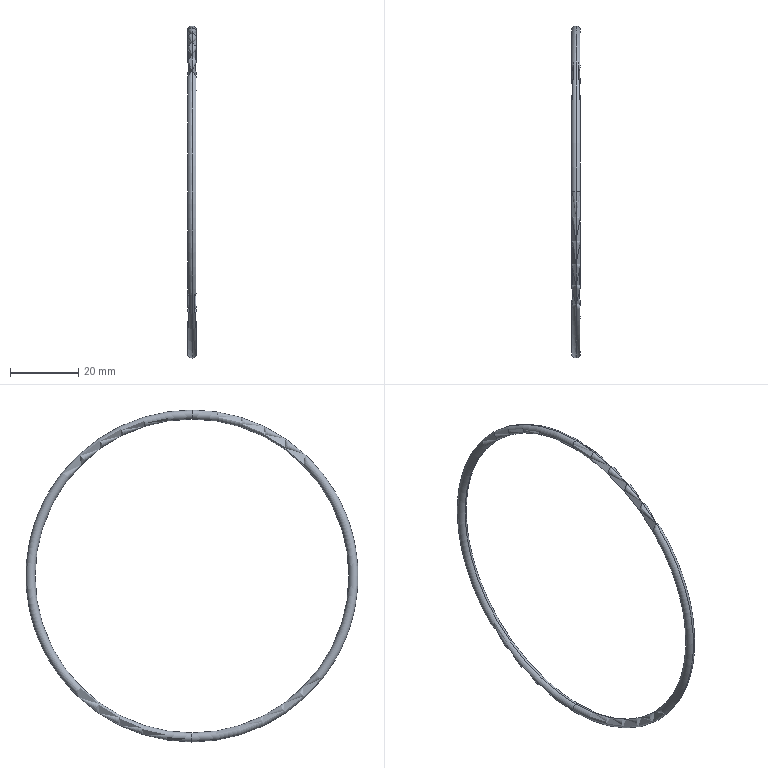Part | SolidWorks | features Revolution 1 | 1 solid | 4 faces | box 2.65 x 97.35 x 97.35 mm | volume 1641 mm3 | torus 4
STEP:
#1=CARTESIAN_POINT('',(5.,0.,-48.675));
#2=VERTEX_POINT('',#1);
#3=CARTESIAN_POINT('',(5.,0.,-46.025));
#4=VERTEX_POINT('',#3);
#5=CARTESIAN_POINT('',(5.,0.,-47.35));
#6=DIRECTION('',(0.,1.,0.));
#7=DIRECTION('',(0.,0.,1.));
#8=AXIS2_PLACEMENT_3D('',#5,#6,#7);
#9=CIRCLE('',#8,1.325);
#10=EDGE_CURVE('',#2,#4,#9,.T.);
#11=ORIENTED_EDGE('',*,*,#10,.F.);
#12=CARTESIAN_POINT('',(5.,0.,48.675));
#13=VERTEX_POINT('',#12);
#14=CARTESIAN_POINT('',(5.,0.,0.));
#15=DIRECTION('',(-1.,0.,0.));
#16=DIRECTION('',(0.,0.,1.));
#17=AXIS2_PLACEMENT_3D('',#14,#15,#16);
#18=CIRCLE('',#17,48.675);
#19=EDGE_CURVE('',#2,#13,#18,.T.);
#20=ORIENTED_EDGE('',*,*,#19,.T.);
#21=CARTESIAN_POINT('',(5.,0.,46.025));
#22=VERTEX_POINT('',#21);
#23=CARTESIAN_POINT('',(5.,0.,47.35));
#24=DIRECTION('',(0.,-1.,0.));
#25=DIRECTION('',(0.,0.,-1.));
#26=AXIS2_PLACEMENT_3D('',#23,#24,#25);
#27=CIRCLE('',#26,1.325);
#28=EDGE_CURVE('',#13,#22,#27,.T.);
#29=ORIENTED_EDGE('',*,*,#28,.T.);
#30=CARTESIAN_POINT('',(5.,0.,0.));
#31=DIRECTION('',(-1.,0.,0.));
#32=DIRECTION('',(0.,0.,1.));
#33=AXIS2_PLACEMENT_3D('',#30,#31,#32);
#34=CIRCLE('',#33,46.025);
#35=EDGE_CURVE('',#4,#22,#34,.T.);
#36=ORIENTED_EDGE('',*,*,#35,.F.);
#37=EDGE_LOOP('',(#11,#20,#29,#36));
#38=FACE_OUTER_BOUND('',#37,.T.);
#39=CARTESIAN_POINT('',(5.,0.,0.));
#40=DIRECTION('',(-1.,0.,0.));
#41=DIRECTION('',(0.,0.,1.));
#42=AXIS2_PLACEMENT_3D('',#39,#40,#41);
#43=TOROIDAL_SURFACE('',#42,47.35,1.325);
#44=ADVANCED_FACE('',(#38),#43,.T.);
#45=ORIENTED_EDGE('',*,*,#28,.F.);
#46=CARTESIAN_POINT('',(5.,0.,0.));
#47=DIRECTION('',(-1.,0.,0.));
#48=DIRECTION('',(0.,0.,1.));
#49=AXIS2_PLACEMENT_3D('',#46,#47,#48);
#50=CIRCLE('',#49,48.675);
#51=EDGE_CURVE('',#13,#2,#50,.T.);
#52=ORIENTED_EDGE('',*,*,#51,.T.);
#53=ORIENTED_EDGE('',*,*,#10,.T.);
#54=CARTESIAN_POINT('',(5.,0.,0.));
#55=DIRECTION('',(-1.,0.,0.));
#56=DIRECTION('',(0.,0.,1.));
#57=AXIS2_PLACEMENT_3D('',#54,#55,#56);
#58=CIRCLE('',#57,46.025);
#59=EDGE_CURVE('',#22,#4,#58,.T.);
#60=ORIENTED_EDGE('',*,*,#59,.F.);
#61=EDGE_LOOP('',(#45,#52,#53,#60));
#62=FACE_OUTER_BOUND('',#61,.T.);
#63=CARTESIAN_POINT('',(5.,0.,0.));
#64=DIRECTION('',(-1.,0.,0.));
#65=DIRECTION('',(0.,0.,1.));
#66=AXIS2_PLACEMENT_3D('',#63,#64,#65);
#67=TOROIDAL_SURFACE('',#66,47.35,1.325);
#68=ADVANCED_FACE('',(#62),#67,.T.);
#69=ORIENTED_EDGE('',*,*,#51,.F.);
#70=CARTESIAN_POINT('',(5.,0.,47.35));
#71=DIRECTION('',(0.,-1.,0.));
#72=DIRECTION('',(0.,0.,-1.));
#73=AXIS2_PLACEMENT_3D('',#70,#71,#72);
#74=CIRCLE('',#73,1.325);
#75=EDGE_CURVE('',#22,#13,#74,.T.);
#76=ORIENTED_EDGE('',*,*,#75,.F.);
#77=ORIENTED_EDGE('',*,*,#59,.T.);
#78=CARTESIAN_POINT('',(5.,0.,-47.35));
#79=DIRECTION('',(0.,1.,0.));
#80=DIRECTION('',(0.,0.,1.));
#81=AXIS2_PLACEMENT_3D('',#78,#79,#80);
#82=CIRCLE('',#81,1.325);
#83=EDGE_CURVE('',#4,#2,#82,.T.);
#84=ORIENTED_EDGE('',*,*,#83,.T.);
#85=EDGE_LOOP('',(#69,#76,#77,#84));
#86=FACE_OUTER_BOUND('',#85,.T.);
#87=CARTESIAN_POINT('',(5.,0.,0.));
#88=DIRECTION('',(-1.,0.,0.));
#89=DIRECTION('',(0.,0.,1.));
#90=AXIS2_PLACEMENT_3D('',#87,#88,#89);
#91=TOROIDAL_SURFACE('',#90,47.35,1.325);
#92=ADVANCED_FACE('',(#86),#91,.T.);
#93=ORIENTED_EDGE('',*,*,#19,.F.);
#94=ORIENTED_EDGE('',*,*,#83,.F.);
#95=ORIENTED_EDGE('',*,*,#35,.T.);
#96=ORIENTED_EDGE('',*,*,#75,.T.);
#97=EDGE_LOOP('',(#93,#94,#95,#96));
#98=FACE_OUTER_BOUND('',#97,.T.);
#99=CARTESIAN_POINT('',(5.,0.,0.));
#100=DIRECTION('',(-1.,0.,0.));
#101=DIRECTION('',(0.,0.,1.));
#102=AXIS2_PLACEMENT_3D('',#99,#100,#101);
#103=TOROIDAL_SURFACE('',#102,47.35,1.325);
#104=ADVANCED_FACE('',(#98),#103,.T.);
#105=CLOSED_SHELL('',(#44,#68,#92,#104));
#106=MANIFOLD_SOLID_BREP('',#105);
#107=CARTESIAN_POINT('',(0.,0.,0.));
#108=DIRECTION('',(0.,0.,1.));
#109=DIRECTION('',(1.,0.,0.));
#110=AXIS2_PLACEMENT_3D('',#107,#108,#109);
#111=(LENGTH_UNIT()NAMED_UNIT(*)SI_UNIT(.MILLI.,.METRE.));
#112=UNCERTAINTY_MEASURE_WITH_UNIT(LENGTH_MEASURE(0.00001),#111,'','');
#113=(NAMED_UNIT(*)PLANE_ANGLE_UNIT()SI_UNIT($,.RADIAN.));
#114=(NAMED_UNIT(*)SI_UNIT($,.STERADIAN.)SOLID_ANGLE_UNIT());
#115=(GEOMETRIC_REPRESENTATION_CONTEXT(3)GLOBAL_UNCERTAINTY_ASSIGNED_CONTEXT((#112))GLOBAL_UNIT_ASSIGNED_CONTEXT((#111,#113,#114))REPRESENTATION_CONTEXT('',''));
#116=ADVANCED_BREP_SHAPE_REPRESENTATION('',(#106,#110),#115);